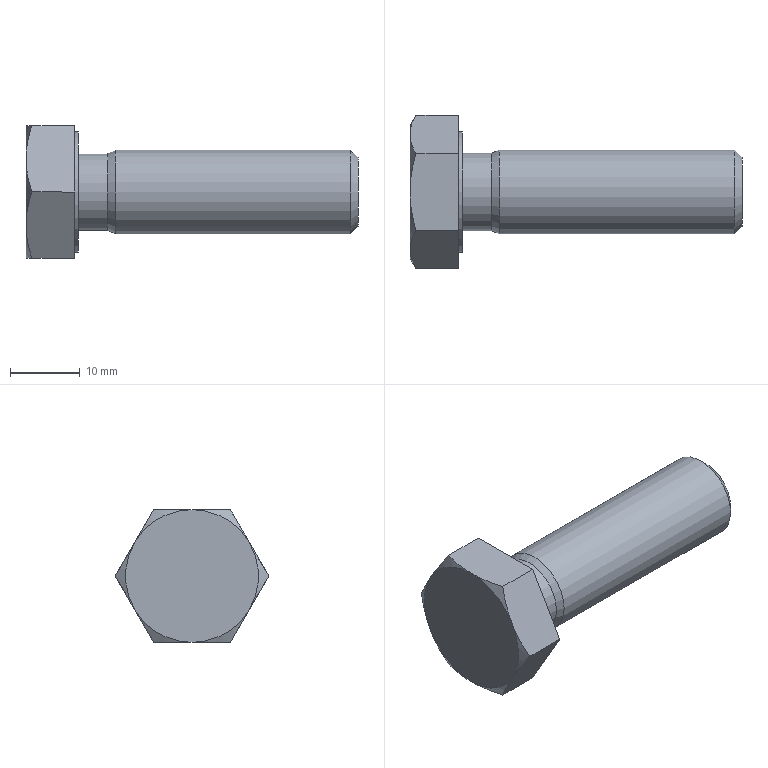Part | STEP file | DIN 933 - M12  x 40 | 1 solid | 21 faces | box 47.5 x 21.939 x 19 mm | volume 6712 mm3 | plane 10 | cone 8 | cylinder 3 | commonest cylinder face diameters 11.053 x1 12 x1 17.2 x1